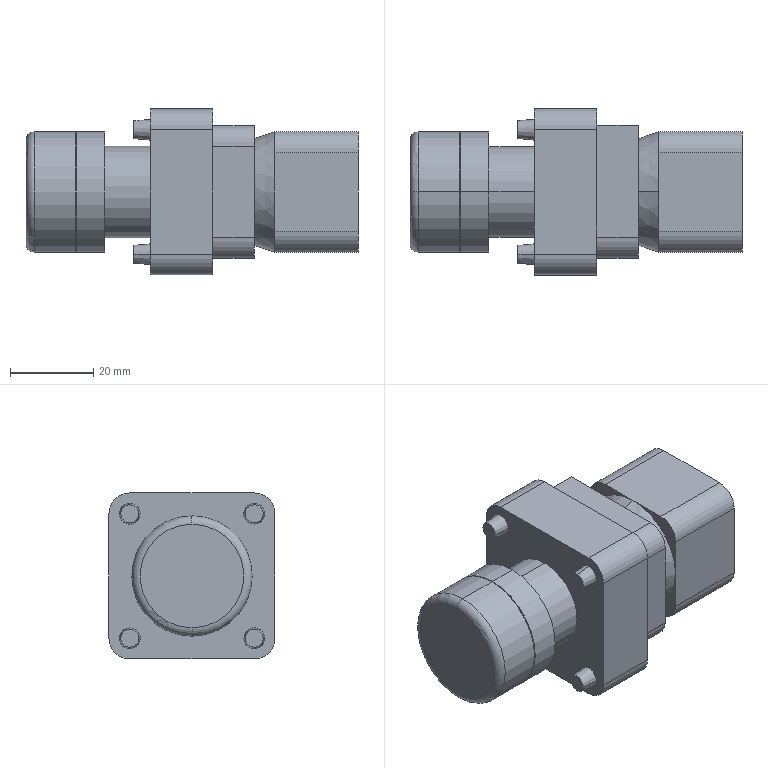Part | SolidWorks | features BaseBody 1 | 1 solid | 59 faces | box 80 x 40 x 40 mm | volume 70018 mm3 | plane 28 | cylinder 19 | cone 10 | torus 2 | commonest cylinder face diameters 10 x11 29 x4 22 x2 28.6 x2